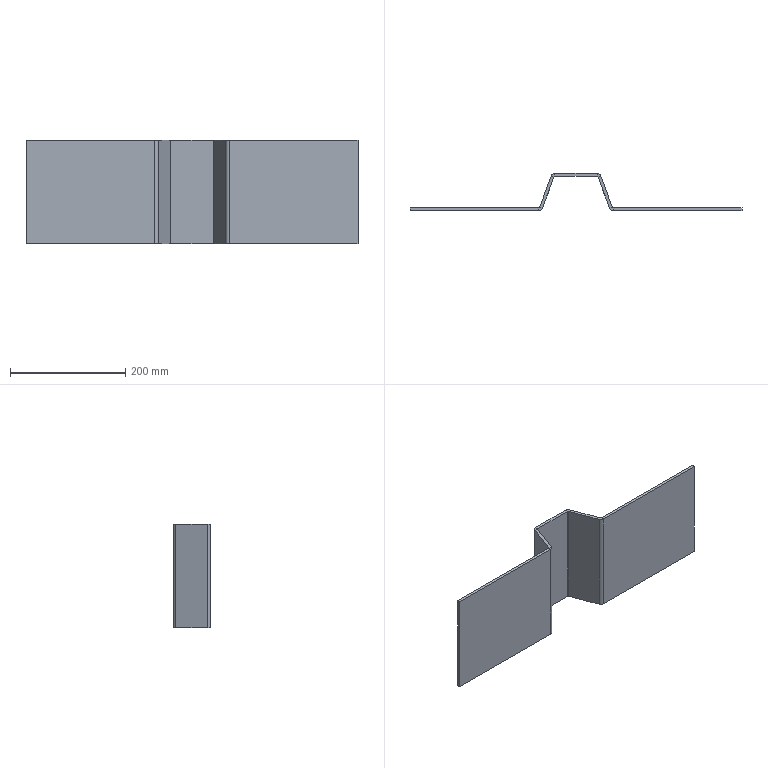Part | STEP file | Tube-changer housing base plate SGN-2-01-002 | 1 solid | 38 faces | box 575 x 65 x 180 mm | volume 589839 mm3 | plane 30 | cylinder 8 | commonest cylinder face diameters 3 x4 13 x4